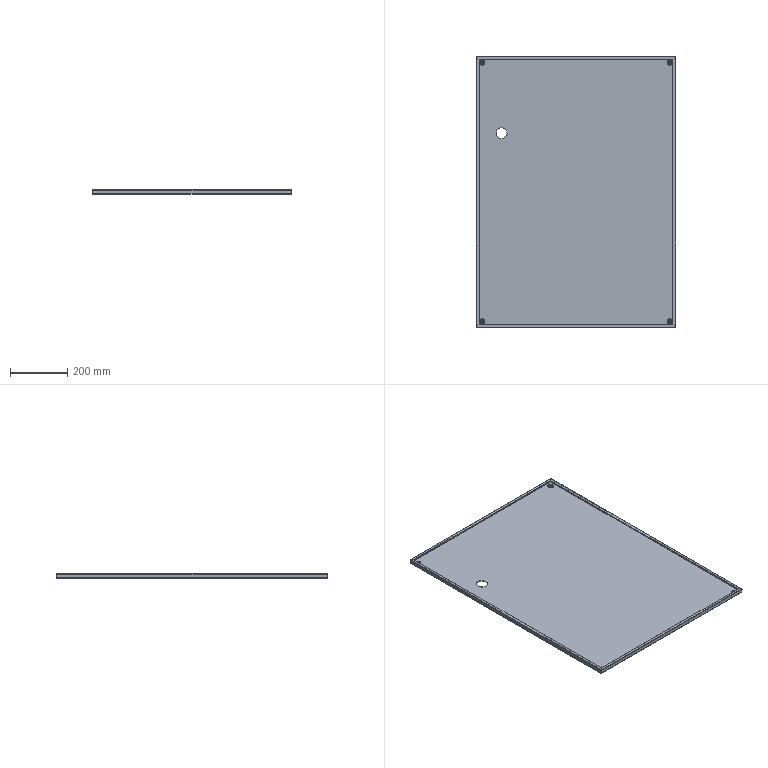Part | STEP file | HESS-408-70-15W-W-10-outer case rear closing plate | 1 solid | 136 faces | box 697 x 947 x 15 mm | volume 1092654 mm3 | spline 48 | plane 46 | cylinder 26 | cone 16 | commonest cylinder face diameters 0.2 x8 3.2 x8 5 x8 38 x2